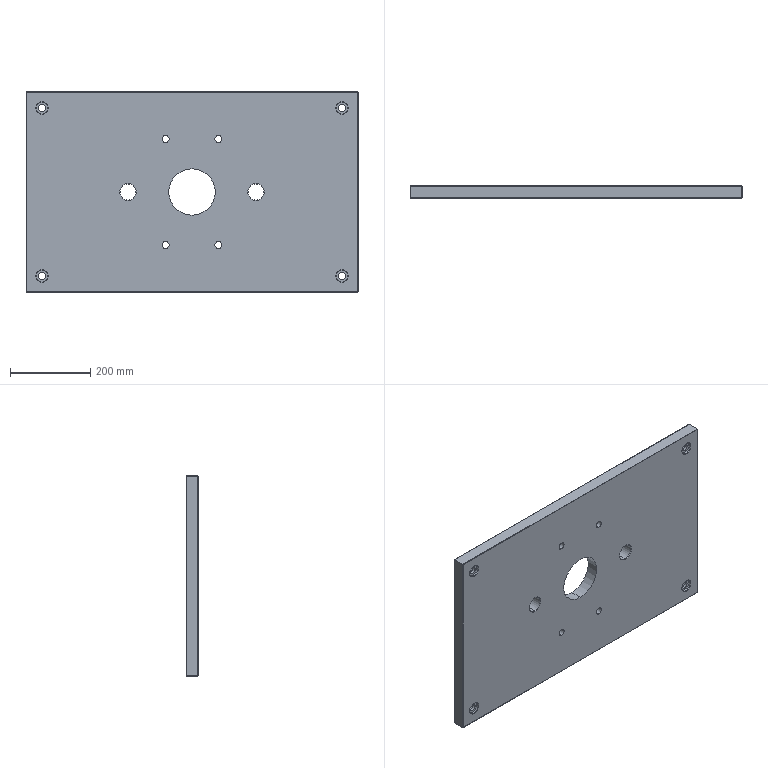Part | STEP file | OP10-015_upper plate (R) | 1 solid | 120 faces | box 830 x 30 x 500 mm | volume 11965726 mm3 | cylinder 54 | plane 34 | cone 32 | commonest cylinder face diameters 4.2 x16 17.5 x8 18 x8 26 x8 30 x8 40 x4